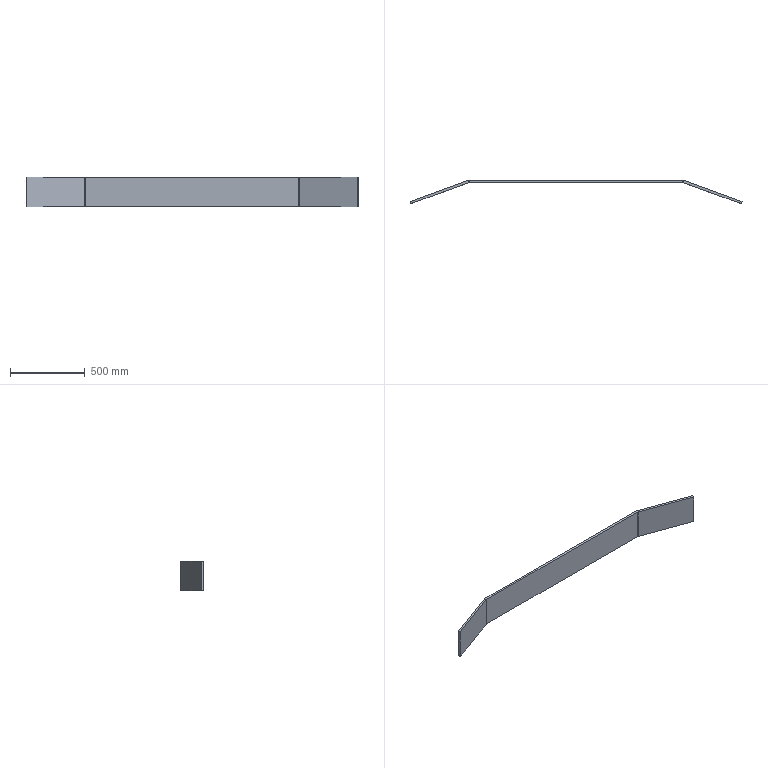Part | SolidWorks | features FlatPattern 1, SMBaseFlange 1, SheetMetal 1 | 1 solid | 22 faces | box 2215 x 156.912 x 200 mm | volume 7230328 mm3 | plane 18 | cylinder 4 | commonest cylinder face diameters 30 x2 62 x2
STEP:
#1=CARTESIAN_POINT('',(-717.485,-0.9046,200.));
#2=VERTEX_POINT('',#1);
#3=CARTESIAN_POINT('',(-722.958,14.13,200.));
#4=VERTEX_POINT('',#3);
#5=CARTESIAN_POINT('',(-717.485,-0.9046,200.));
#6=DIRECTION('',(-0.342,0.9397,0.));
#7=VECTOR('',#6,1000.);
#8=LINE('',#5,#7);
#9=EDGE_CURVE('',#2,#4,#8,.T.);
#10=ORIENTED_EDGE('',*,*,#9,.F.);
#11=CARTESIAN_POINT('',(-712.355,0.,200.));
#12=VERTEX_POINT('',#11);
#13=CARTESIAN_POINT('',(-712.355,-15.,200.));
#14=DIRECTION('',(0.,0.,-1.));
#15=DIRECTION('',(1.,0.,0.));
#16=AXIS2_PLACEMENT_3D('',#13,#14,#15);
#17=CIRCLE('',#16,15.);
#18=EDGE_CURVE('',#2,#12,#17,.T.);
#19=ORIENTED_EDGE('',*,*,#18,.T.);
#20=CARTESIAN_POINT('',(-712.355,16.,200.));
#21=VERTEX_POINT('',#20);
#22=CARTESIAN_POINT('',(-712.355,16.,200.));
#23=DIRECTION('',(0.,-1.,0.));
#24=VECTOR('',#23,1000.);
#25=LINE('',#22,#24);
#26=EDGE_CURVE('',#21,#12,#25,.T.);
#27=ORIENTED_EDGE('',*,*,#26,.F.);
#28=CARTESIAN_POINT('',(-712.355,-15.,200.));
#29=DIRECTION('',(0.,0.,-1.));
#30=DIRECTION('',(1.,0.,0.));
#31=AXIS2_PLACEMENT_3D('',#28,#29,#30);
#32=CIRCLE('',#31,31.);
#33=EDGE_CURVE('',#4,#21,#32,.T.);
#34=ORIENTED_EDGE('',*,*,#33,.F.);
#35=EDGE_LOOP('',(#10,#19,#27,#34));
#36=FACE_OUTER_BOUND('',#35,.T.);
#37=CARTESIAN_POINT('',(-717.485,-0.9046,200.));
#38=DIRECTION('',(0.,0.,1.));
#39=DIRECTION('',(1.,0.,0.));
#40=AXIS2_PLACEMENT_3D('',#37,#38,#39);
#41=PLANE('',#40);
#42=ADVANCED_FACE('',(#36),#41,.T.);
#43=CARTESIAN_POINT('',(-1102.153,-140.912,200.));
#44=VERTEX_POINT('',#43);
#45=CARTESIAN_POINT('',(-715.,0.,200.));
#46=DIRECTION('',(0.9397,0.342,0.));
#47=VECTOR('',#46,1000.);
#48=LINE('',#45,#47);
#49=EDGE_CURVE('',#44,#2,#48,.T.);
#50=ORIENTED_EDGE('',*,*,#49,.T.);
#51=ORIENTED_EDGE('',*,*,#9,.T.);
#52=CARTESIAN_POINT('',(-1107.626,-125.877,200.));
#53=VERTEX_POINT('',#52);
#54=CARTESIAN_POINT('',(-720.472,15.035,200.));
#55=DIRECTION('',(0.9397,0.342,0.));
#56=VECTOR('',#55,1000.);
#57=LINE('',#54,#56);
#58=EDGE_CURVE('',#53,#4,#57,.T.);
#59=ORIENTED_EDGE('',*,*,#58,.F.);
#60=CARTESIAN_POINT('',(-1102.153,-140.912,200.));
#61=DIRECTION('',(-0.342,0.9397,0.));
#62=VECTOR('',#61,1000.);
#63=LINE('',#60,#62);
#64=EDGE_CURVE('',#44,#53,#63,.T.);
#65=ORIENTED_EDGE('',*,*,#64,.F.);
#66=EDGE_LOOP('',(#50,#51,#59,#65));
#67=FACE_OUTER_BOUND('',#66,.T.);
#68=CARTESIAN_POINT('',(-712.355,16.,200.));
#69=DIRECTION('',(0.,0.,1.));
#70=DIRECTION('',(1.,0.,0.));
#71=AXIS2_PLACEMENT_3D('',#68,#69,#70);
#72=PLANE('',#71);
#73=ADVANCED_FACE('',(#67),#72,.T.);
#74=CARTESIAN_POINT('',(-712.355,0.,0.));
#75=VERTEX_POINT('',#74);
#76=CARTESIAN_POINT('',(-712.355,16.,0.));
#77=VERTEX_POINT('',#76);
#78=CARTESIAN_POINT('',(-712.355,0.,0.));
#79=DIRECTION('',(0.,1.,0.));
#80=VECTOR('',#79,1000.);
#81=LINE('',#78,#80);
#82=EDGE_CURVE('',#75,#77,#81,.T.);
#83=ORIENTED_EDGE('',*,*,#82,.F.);
#84=CARTESIAN_POINT('',(-717.485,-0.9046,0.));
#85=VERTEX_POINT('',#84);
#86=CARTESIAN_POINT('',(-712.355,-15.,0.));
#87=DIRECTION('',(0.,0.,-1.));
#88=DIRECTION('',(1.,0.,0.));
#89=AXIS2_PLACEMENT_3D('',#86,#87,#88);
#90=CIRCLE('',#89,15.);
#91=EDGE_CURVE('',#85,#75,#90,.T.);
#92=ORIENTED_EDGE('',*,*,#91,.F.);
#93=CARTESIAN_POINT('',(-722.958,14.13,0.));
#94=VERTEX_POINT('',#93);
#95=CARTESIAN_POINT('',(-722.958,14.13,0.));
#96=DIRECTION('',(0.342,-0.9397,0.));
#97=VECTOR('',#96,1000.);
#98=LINE('',#95,#97);
#99=EDGE_CURVE('',#94,#85,#98,.T.);
#100=ORIENTED_EDGE('',*,*,#99,.F.);
#101=CARTESIAN_POINT('',(-712.355,-15.,0.));
#102=DIRECTION('',(0.,0.,-1.));
#103=DIRECTION('',(1.,0.,0.));
#104=AXIS2_PLACEMENT_3D('',#101,#102,#103);
#105=CIRCLE('',#104,31.);
#106=EDGE_CURVE('',#94,#77,#105,.T.);
#107=ORIENTED_EDGE('',*,*,#106,.T.);
#108=EDGE_LOOP('',(#83,#92,#100,#107));
#109=FACE_OUTER_BOUND('',#108,.T.);
#110=CARTESIAN_POINT('',(-712.355,0.,0.));
#111=DIRECTION('',(0.,0.,-1.));
#112=DIRECTION('',(-1.,0.,0.));
#113=AXIS2_PLACEMENT_3D('',#110,#111,#112);
#114=PLANE('',#113);
#115=ADVANCED_FACE('',(#109),#114,.T.);
#116=CARTESIAN_POINT('',(712.355,0.,0.));
#117=VERTEX_POINT('',#116);
#118=CARTESIAN_POINT('',(-715.,0.,0.));
#119=DIRECTION('',(1.,0.,0.));
#120=VECTOR('',#119,1000.);
#121=LINE('',#118,#120);
#122=EDGE_CURVE('',#75,#117,#121,.T.);
#123=ORIENTED_EDGE('',*,*,#122,.F.);
#124=ORIENTED_EDGE('',*,*,#82,.T.);
#125=CARTESIAN_POINT('',(712.355,16.,0.));
#126=VERTEX_POINT('',#125);
#127=CARTESIAN_POINT('',(-715.,16.,0.));
#128=DIRECTION('',(1.,0.,0.));
#129=VECTOR('',#128,1000.);
#130=LINE('',#127,#129);
#131=EDGE_CURVE('',#77,#126,#130,.T.);
#132=ORIENTED_EDGE('',*,*,#131,.T.);
#133=CARTESIAN_POINT('',(712.355,16.,0.));
#134=DIRECTION('',(0.,-1.,0.));
#135=VECTOR('',#134,1000.);
#136=LINE('',#133,#135);
#137=EDGE_CURVE('',#126,#117,#136,.T.);
#138=ORIENTED_EDGE('',*,*,#137,.T.);
#139=EDGE_LOOP('',(#123,#124,#132,#138));
#140=FACE_OUTER_BOUND('',#139,.T.);
#141=CARTESIAN_POINT('',(-722.958,14.13,0.));
#142=DIRECTION('',(0.,0.,-1.));
#143=DIRECTION('',(-1.,0.,0.));
#144=AXIS2_PLACEMENT_3D('',#141,#142,#143);
#145=PLANE('',#144);
#146=ADVANCED_FACE('',(#140),#145,.T.);
#147=CARTESIAN_POINT('',(712.355,0.,200.));
#148=VERTEX_POINT('',#147);
#149=CARTESIAN_POINT('',(712.355,16.,200.));
#150=VERTEX_POINT('',#149);
#151=CARTESIAN_POINT('',(712.355,0.,200.));
#152=DIRECTION('',(0.,1.,0.));
#153=VECTOR('',#152,1000.);
#154=LINE('',#151,#153);
#155=EDGE_CURVE('',#148,#150,#154,.T.);
#156=ORIENTED_EDGE('',*,*,#155,.F.);
#157=CARTESIAN_POINT('',(717.485,-0.9046,200.));
#158=VERTEX_POINT('',#157);
#159=CARTESIAN_POINT('',(712.355,-15.,200.));
#160=DIRECTION('',(0.,0.,-1.));
#161=DIRECTION('',(1.,0.,0.));
#162=AXIS2_PLACEMENT_3D('',#159,#160,#161);
#163=CIRCLE('',#162,15.);
#164=EDGE_CURVE('',#148,#158,#163,.T.);
#165=ORIENTED_EDGE('',*,*,#164,.T.);
#166=CARTESIAN_POINT('',(722.958,14.13,200.));
#167=VERTEX_POINT('',#166);
#168=CARTESIAN_POINT('',(722.958,14.13,200.));
#169=DIRECTION('',(-0.342,-0.9397,0.));
#170=VECTOR('',#169,1000.);
#171=LINE('',#168,#170);
#172=EDGE_CURVE('',#167,#158,#171,.T.);
#173=ORIENTED_EDGE('',*,*,#172,.F.);
#174=CARTESIAN_POINT('',(712.355,-15.,200.));
#175=DIRECTION('',(0.,0.,-1.));
#176=DIRECTION('',(1.,0.,0.));
#177=AXIS2_PLACEMENT_3D('',#174,#175,#176);
#178=CIRCLE('',#177,31.);
#179=EDGE_CURVE('',#150,#167,#178,.T.);
#180=ORIENTED_EDGE('',*,*,#179,.F.);
#181=EDGE_LOOP('',(#156,#165,#173,#180));
#182=FACE_OUTER_BOUND('',#181,.T.);
#183=CARTESIAN_POINT('',(712.355,0.,200.));
#184=DIRECTION('',(0.,0.,1.));
#185=DIRECTION('',(1.,0.,0.));
#186=AXIS2_PLACEMENT_3D('',#183,#184,#185);
#187=PLANE('',#186);
#188=ADVANCED_FACE('',(#182),#187,.T.);
#189=CARTESIAN_POINT('',(-715.,0.,200.));
#190=DIRECTION('',(1.,0.,0.));
#191=VECTOR('',#190,1000.);
#192=LINE('',#189,#191);
#193=EDGE_CURVE('',#12,#148,#192,.T.);
#194=ORIENTED_EDGE('',*,*,#193,.T.);
#195=ORIENTED_EDGE('',*,*,#155,.T.);
#196=CARTESIAN_POINT('',(-715.,16.,200.));
#197=DIRECTION('',(1.,0.,0.));
#198=VECTOR('',#197,1000.);
#199=LINE('',#196,#198);
#200=EDGE_CURVE('',#21,#150,#199,.T.);
#201=ORIENTED_EDGE('',*,*,#200,.F.);
#202=ORIENTED_EDGE('',*,*,#26,.T.);
#203=EDGE_LOOP('',(#194,#195,#201,#202));
#204=FACE_OUTER_BOUND('',#203,.T.);
#205=CARTESIAN_POINT('',(722.958,14.13,200.));
#206=DIRECTION('',(0.,0.,1.));
#207=DIRECTION('',(1.,0.,0.));
#208=AXIS2_PLACEMENT_3D('',#205,#206,#207);
#209=PLANE('',#208);
#210=ADVANCED_FACE('',(#204),#209,.T.);
#211=CARTESIAN_POINT('',(717.485,-0.9046,0.));
#212=VERTEX_POINT('',#211);
#213=CARTESIAN_POINT('',(722.958,14.13,0.));
#214=VERTEX_POINT('',#213);
#215=CARTESIAN_POINT('',(717.485,-0.9046,0.));
#216=DIRECTION('',(0.342,0.9397,0.));
#217=VECTOR('',#216,1000.);
#218=LINE('',#215,#217);
#219=EDGE_CURVE('',#212,#214,#218,.T.);
#220=ORIENTED_EDGE('',*,*,#219,.F.);
#221=CARTESIAN_POINT('',(712.355,-15.,0.));
#222=DIRECTION('',(0.,0.,-1.));
#223=DIRECTION('',(1.,0.,0.));
#224=AXIS2_PLACEMENT_3D('',#221,#222,#223);
#225=CIRCLE('',#224,15.);
#226=EDGE_CURVE('',#117,#212,#225,.T.);
#227=ORIENTED_EDGE('',*,*,#226,.F.);
#228=ORIENTED_EDGE('',*,*,#137,.F.);
#229=CARTESIAN_POINT('',(712.355,-15.,0.));
#230=DIRECTION('',(0.,0.,-1.));
#231=DIRECTION('',(1.,0.,0.));
#232=AXIS2_PLACEMENT_3D('',#229,#230,#231);
#233=CIRCLE('',#232,31.);
#234=EDGE_CURVE('',#126,#214,#233,.T.);
#235=ORIENTED_EDGE('',*,*,#234,.T.);
#236=EDGE_LOOP('',(#220,#227,#228,#235));
#237=FACE_OUTER_BOUND('',#236,.T.);
#238=CARTESIAN_POINT('',(717.485,-0.9046,0.));
#239=DIRECTION('',(0.,0.,-1.));
#240=DIRECTION('',(-1.,0.,0.));
#241=AXIS2_PLACEMENT_3D('',#238,#239,#240);
#242=PLANE('',#241);
#243=ADVANCED_FACE('',(#237),#242,.T.);
#244=CARTESIAN_POINT('',(1102.153,-140.912,0.));
#245=VERTEX_POINT('',#244);
#246=CARTESIAN_POINT('',(715.,0.,0.));
#247=DIRECTION('',(0.9397,-0.342,0.));
#248=VECTOR('',#247,1000.);
#249=LINE('',#246,#248);
#250=EDGE_CURVE('',#212,#245,#249,.T.);
#251=ORIENTED_EDGE('',*,*,#250,.F.);
#252=ORIENTED_EDGE('',*,*,#219,.T.);
#253=CARTESIAN_POINT('',(1107.626,-125.877,0.));
#254=VERTEX_POINT('',#253);
#255=CARTESIAN_POINT('',(720.472,15.035,0.));
#256=DIRECTION('',(0.9397,-0.342,0.));
#257=VECTOR('',#256,1000.);
#258=LINE('',#255,#257);
#259=EDGE_CURVE('',#214,#254,#258,.T.);
#260=ORIENTED_EDGE('',*,*,#259,.T.);
#261=CARTESIAN_POINT('',(1107.626,-125.877,0.));
#262=DIRECTION('',(-0.342,-0.9397,0.));
#263=VECTOR('',#262,1000.);
#264=LINE('',#261,#263);
#265=EDGE_CURVE('',#254,#245,#264,.T.);
#266=ORIENTED_EDGE('',*,*,#265,.T.);
#267=EDGE_LOOP('',(#251,#252,#260,#266));
#268=FACE_OUTER_BOUND('',#267,.T.);
#269=CARTESIAN_POINT('',(712.355,16.,0.));
#270=DIRECTION('',(0.,0.,-1.));
#271=DIRECTION('',(-1.,0.,0.));
#272=AXIS2_PLACEMENT_3D('',#269,#270,#271);
#273=PLANE('',#272);
#274=ADVANCED_FACE('',(#268),#273,.T.);
#275=ORIENTED_EDGE('',*,*,#250,.T.);
#276=CARTESIAN_POINT('',(1102.153,-140.912,200.));
#277=VERTEX_POINT('',#276);
#278=CARTESIAN_POINT('',(1102.153,-140.912,200.));
#279=DIRECTION('',(0.,0.,-1.));
#280=VECTOR('',#279,1000.);
#281=LINE('',#278,#280);
#282=EDGE_CURVE('',#277,#245,#281,.T.);
#283=ORIENTED_EDGE('',*,*,#282,.F.);
#284=CARTESIAN_POINT('',(715.,0.,200.));
#285=DIRECTION('',(0.9397,-0.342,0.));
#286=VECTOR('',#285,1000.);
#287=LINE('',#284,#286);
#288=EDGE_CURVE('',#158,#277,#287,.T.);
#289=ORIENTED_EDGE('',*,*,#288,.F.);
#290=CARTESIAN_POINT('',(717.485,-0.9046,200.));
#291=DIRECTION('',(0.,0.,-1.));
#292=VECTOR('',#291,1000.);
#293=LINE('',#290,#292);
#294=EDGE_CURVE('',#158,#212,#293,.T.);
#295=ORIENTED_EDGE('',*,*,#294,.T.);
#296=EDGE_LOOP('',(#275,#283,#289,#295));
#297=FACE_OUTER_BOUND('',#296,.T.);
#298=CARTESIAN_POINT('',(715.,0.,200.));
#299=DIRECTION('',(0.342,0.9397,0.));
#300=DIRECTION('',(-0.9397,0.342,0.));
#301=AXIS2_PLACEMENT_3D('',#298,#299,#300);
#302=PLANE('',#301);
#303=ADVANCED_FACE('',(#297),#302,.F.);
#304=ORIENTED_EDGE('',*,*,#265,.F.);
#305=CARTESIAN_POINT('',(1107.626,-125.877,200.));
#306=VERTEX_POINT('',#305);
#307=CARTESIAN_POINT('',(1107.626,-125.877,200.));
#308=DIRECTION('',(0.,0.,-1.));
#309=VECTOR('',#308,1000.);
#310=LINE('',#307,#309);
#311=EDGE_CURVE('',#306,#254,#310,.T.);
#312=ORIENTED_EDGE('',*,*,#311,.F.);
#313=CARTESIAN_POINT('',(1107.626,-125.877,200.));
#314=DIRECTION('',(-0.342,-0.9397,0.));
#315=VECTOR('',#314,1000.);
#316=LINE('',#313,#315);
#317=EDGE_CURVE('',#306,#277,#316,.T.);
#318=ORIENTED_EDGE('',*,*,#317,.T.);
#319=ORIENTED_EDGE('',*,*,#282,.T.);
#320=EDGE_LOOP('',(#304,#312,#318,#319));
#321=FACE_OUTER_BOUND('',#320,.T.);
#322=CARTESIAN_POINT('',(1107.626,-125.877,200.));
#323=DIRECTION('',(0.9397,-0.342,0.));
#324=DIRECTION('',(0.342,0.9397,0.));
#325=AXIS2_PLACEMENT_3D('',#322,#323,#324);
#326=PLANE('',#325);
#327=ADVANCED_FACE('',(#321),#326,.T.);
#328=ORIENTED_EDGE('',*,*,#259,.F.);
#329=CARTESIAN_POINT('',(722.958,14.13,200.));
#330=DIRECTION('',(0.,0.,-1.));
#331=VECTOR('',#330,1000.);
#332=LINE('',#329,#331);
#333=EDGE_CURVE('',#167,#214,#332,.T.);
#334=ORIENTED_EDGE('',*,*,#333,.F.);
#335=CARTESIAN_POINT('',(720.472,15.035,200.));
#336=DIRECTION('',(0.9397,-0.342,0.));
#337=VECTOR('',#336,1000.);
#338=LINE('',#335,#337);
#339=EDGE_CURVE('',#167,#306,#338,.T.);
#340=ORIENTED_EDGE('',*,*,#339,.T.);
#341=ORIENTED_EDGE('',*,*,#311,.T.);
#342=EDGE_LOOP('',(#328,#334,#340,#341));
#343=FACE_OUTER_BOUND('',#342,.T.);
#344=CARTESIAN_POINT('',(720.472,15.035,200.));
#345=DIRECTION('',(0.342,0.9397,0.));
#346=DIRECTION('',(-0.9397,0.342,0.));
#347=AXIS2_PLACEMENT_3D('',#344,#345,#346);
#348=PLANE('',#347);
#349=ADVANCED_FACE('',(#343),#348,.T.);
#350=ORIENTED_EDGE('',*,*,#234,.F.);
#351=CARTESIAN_POINT('',(712.355,16.,200.));
#352=DIRECTION('',(0.,0.,-1.));
#353=VECTOR('',#352,1000.);
#354=LINE('',#351,#353);
#355=EDGE_CURVE('',#150,#126,#354,.T.);
#356=ORIENTED_EDGE('',*,*,#355,.F.);
#357=ORIENTED_EDGE('',*,*,#179,.T.);
#358=ORIENTED_EDGE('',*,*,#333,.T.);
#359=EDGE_LOOP('',(#350,#356,#357,#358));
#360=FACE_OUTER_BOUND('',#359,.T.);
#361=CARTESIAN_POINT('',(712.355,-15.,200.));
#362=DIRECTION('',(0.,0.,-1.));
#363=DIRECTION('',(-1.,0.,0.));
#364=AXIS2_PLACEMENT_3D('',#361,#362,#363);
#365=CYLINDRICAL_SURFACE('',#364,31.);
#366=ADVANCED_FACE('',(#360),#365,.T.);
#367=ORIENTED_EDGE('',*,*,#131,.F.);
#368=CARTESIAN_POINT('',(-712.355,16.,200.));
#369=DIRECTION('',(0.,0.,-1.));
#370=VECTOR('',#369,1000.);
#371=LINE('',#368,#370);
#372=EDGE_CURVE('',#21,#77,#371,.T.);
#373=ORIENTED_EDGE('',*,*,#372,.F.);
#374=ORIENTED_EDGE('',*,*,#200,.T.);
#375=ORIENTED_EDGE('',*,*,#355,.T.);
#376=EDGE_LOOP('',(#367,#373,#374,#375));
#377=FACE_OUTER_BOUND('',#376,.T.);
#378=CARTESIAN_POINT('',(-715.,16.,200.));
#379=DIRECTION('',(0.,1.,0.));
#380=DIRECTION('',(0.,0.,1.));
#381=AXIS2_PLACEMENT_3D('',#378,#379,#380);
#382=PLANE('',#381);
#383=ADVANCED_FACE('',(#377),#382,.T.);
#384=ORIENTED_EDGE('',*,*,#106,.F.);
#385=CARTESIAN_POINT('',(-722.958,14.13,200.));
#386=DIRECTION('',(0.,0.,-1.));
#387=VECTOR('',#386,1000.);
#388=LINE('',#385,#387);
#389=EDGE_CURVE('',#4,#94,#388,.T.);
#390=ORIENTED_EDGE('',*,*,#389,.F.);
#391=ORIENTED_EDGE('',*,*,#33,.T.);
#392=ORIENTED_EDGE('',*,*,#372,.T.);
#393=EDGE_LOOP('',(#384,#390,#391,#392));
#394=FACE_OUTER_BOUND('',#393,.T.);
#395=CARTESIAN_POINT('',(-712.355,-15.,200.));
#396=DIRECTION('',(0.,0.,-1.));
#397=DIRECTION('',(-1.,0.,0.));
#398=AXIS2_PLACEMENT_3D('',#395,#396,#397);
#399=CYLINDRICAL_SURFACE('',#398,31.);
#400=ADVANCED_FACE('',(#394),#399,.T.);
#401=CARTESIAN_POINT('',(-1107.626,-125.877,0.));
#402=VERTEX_POINT('',#401);
#403=CARTESIAN_POINT('',(-720.472,15.035,0.));
#404=DIRECTION('',(0.9397,0.342,0.));
#405=VECTOR('',#404,1000.);
#406=LINE('',#403,#405);
#407=EDGE_CURVE('',#402,#94,#406,.T.);
#408=ORIENTED_EDGE('',*,*,#407,.F.);
#409=CARTESIAN_POINT('',(-1107.626,-125.877,200.));
#410=DIRECTION('',(0.,0.,-1.));
#411=VECTOR('',#410,1000.);
#412=LINE('',#409,#411);
#413=EDGE_CURVE('',#53,#402,#412,.T.);
#414=ORIENTED_EDGE('',*,*,#413,.F.);
#415=ORIENTED_EDGE('',*,*,#58,.T.);
#416=ORIENTED_EDGE('',*,*,#389,.T.);
#417=EDGE_LOOP('',(#408,#414,#415,#416));
#418=FACE_OUTER_BOUND('',#417,.T.);
#419=CARTESIAN_POINT('',(-720.472,15.035,200.));
#420=DIRECTION('',(-0.342,0.9397,0.));
#421=DIRECTION('',(-0.9397,-0.342,0.));
#422=AXIS2_PLACEMENT_3D('',#419,#420,#421);
#423=PLANE('',#422);
#424=ADVANCED_FACE('',(#418),#423,.T.);
#425=CARTESIAN_POINT('',(-1102.153,-140.912,0.));
#426=VERTEX_POINT('',#425);
#427=CARTESIAN_POINT('',(-1102.153,-140.912,0.));
#428=DIRECTION('',(-0.342,0.9397,0.));
#429=VECTOR('',#428,1000.);
#430=LINE('',#427,#429);
#431=EDGE_CURVE('',#426,#402,#430,.T.);
#432=ORIENTED_EDGE('',*,*,#431,.F.);
#433=CARTESIAN_POINT('',(-1102.153,-140.912,200.));
#434=DIRECTION('',(0.,0.,-1.));
#435=VECTOR('',#434,1000.);
#436=LINE('',#433,#435);
#437=EDGE_CURVE('',#44,#426,#436,.T.);
#438=ORIENTED_EDGE('',*,*,#437,.F.);
#439=ORIENTED_EDGE('',*,*,#64,.T.);
#440=ORIENTED_EDGE('',*,*,#413,.T.);
#441=EDGE_LOOP('',(#432,#438,#439,#440));
#442=FACE_OUTER_BOUND('',#441,.T.);
#443=CARTESIAN_POINT('',(-1102.153,-140.912,200.));
#444=DIRECTION('',(-0.9397,-0.342,0.));
#445=DIRECTION('',(0.342,-0.9397,0.));
#446=AXIS2_PLACEMENT_3D('',#443,#444,#445);
#447=PLANE('',#446);
#448=ADVANCED_FACE('',(#442),#447,.T.);
#449=CARTESIAN_POINT('',(-715.,0.,0.));
#450=DIRECTION('',(0.9397,0.342,0.));
#451=VECTOR('',#450,1000.);
#452=LINE('',#449,#451);
#453=EDGE_CURVE('',#426,#85,#452,.T.);
#454=ORIENTED_EDGE('',*,*,#453,.T.);
#455=CARTESIAN_POINT('',(-717.485,-0.9046,200.));
#456=DIRECTION('',(0.,0.,-1.));
#457=VECTOR('',#456,1000.);
#458=LINE('',#455,#457);
#459=EDGE_CURVE('',#2,#85,#458,.T.);
#460=ORIENTED_EDGE('',*,*,#459,.F.);
#461=ORIENTED_EDGE('',*,*,#49,.F.);
#462=ORIENTED_EDGE('',*,*,#437,.T.);
#463=EDGE_LOOP('',(#454,#460,#461,#462));
#464=FACE_OUTER_BOUND('',#463,.T.);
#465=CARTESIAN_POINT('',(-715.,0.,200.));
#466=DIRECTION('',(-0.342,0.9397,0.));
#467=DIRECTION('',(-0.9397,-0.342,0.));
#468=AXIS2_PLACEMENT_3D('',#465,#466,#467);
#469=PLANE('',#468);
#470=ADVANCED_FACE('',(#464),#469,.F.);
#471=ORIENTED_EDGE('',*,*,#91,.T.);
#472=CARTESIAN_POINT('',(-712.355,0.,200.));
#473=DIRECTION('',(0.,0.,-1.));
#474=VECTOR('',#473,1000.);
#475=LINE('',#472,#474);
#476=EDGE_CURVE('',#12,#75,#475,.T.);
#477=ORIENTED_EDGE('',*,*,#476,.F.);
#478=ORIENTED_EDGE('',*,*,#18,.F.);
#479=ORIENTED_EDGE('',*,*,#459,.T.);
#480=EDGE_LOOP('',(#471,#477,#478,#479));
#481=FACE_OUTER_BOUND('',#480,.T.);
#482=CARTESIAN_POINT('',(-712.355,-15.,200.));
#483=DIRECTION('',(0.,0.,-1.));
#484=DIRECTION('',(-1.,0.,0.));
#485=AXIS2_PLACEMENT_3D('',#482,#483,#484);
#486=CYLINDRICAL_SURFACE('',#485,15.);
#487=ADVANCED_FACE('',(#481),#486,.F.);
#488=ORIENTED_EDGE('',*,*,#122,.T.);
#489=CARTESIAN_POINT('',(712.355,0.,200.));
#490=DIRECTION('',(0.,0.,-1.));
#491=VECTOR('',#490,1000.);
#492=LINE('',#489,#491);
#493=EDGE_CURVE('',#148,#117,#492,.T.);
#494=ORIENTED_EDGE('',*,*,#493,.F.);
#495=ORIENTED_EDGE('',*,*,#193,.F.);
#496=ORIENTED_EDGE('',*,*,#476,.T.);
#497=EDGE_LOOP('',(#488,#494,#495,#496));
#498=FACE_OUTER_BOUND('',#497,.T.);
#499=CARTESIAN_POINT('',(-715.,0.,200.));
#500=DIRECTION('',(0.,1.,0.));
#501=DIRECTION('',(0.,0.,1.));
#502=AXIS2_PLACEMENT_3D('',#499,#500,#501);
#503=PLANE('',#502);
#504=ADVANCED_FACE('',(#498),#503,.F.);
#505=ORIENTED_EDGE('',*,*,#226,.T.);
#506=ORIENTED_EDGE('',*,*,#294,.F.);
#507=ORIENTED_EDGE('',*,*,#164,.F.);
#508=ORIENTED_EDGE('',*,*,#493,.T.);
#509=EDGE_LOOP('',(#505,#506,#507,#508));
#510=FACE_OUTER_BOUND('',#509,.T.);
#511=CARTESIAN_POINT('',(712.355,-15.,200.));
#512=DIRECTION('',(0.,0.,-1.));
#513=DIRECTION('',(-1.,0.,0.));
#514=AXIS2_PLACEMENT_3D('',#511,#512,#513);
#515=CYLINDRICAL_SURFACE('',#514,15.);
#516=ADVANCED_FACE('',(#510),#515,.F.);
#517=ORIENTED_EDGE('',*,*,#288,.T.);
#518=ORIENTED_EDGE('',*,*,#317,.F.);
#519=ORIENTED_EDGE('',*,*,#339,.F.);
#520=ORIENTED_EDGE('',*,*,#172,.T.);
#521=EDGE_LOOP('',(#517,#518,#519,#520));
#522=FACE_OUTER_BOUND('',#521,.T.);
#523=CARTESIAN_POINT('',(712.355,-15.,200.));
#524=DIRECTION('',(0.,0.,1.));
#525=DIRECTION('',(1.,0.,0.));
#526=AXIS2_PLACEMENT_3D('',#523,#524,#525);
#527=PLANE('',#526);
#528=ADVANCED_FACE('',(#522),#527,.T.);
#529=ORIENTED_EDGE('',*,*,#407,.T.);
#530=ORIENTED_EDGE('',*,*,#99,.T.);
#531=ORIENTED_EDGE('',*,*,#453,.F.);
#532=ORIENTED_EDGE('',*,*,#431,.T.);
#533=EDGE_LOOP('',(#529,#530,#531,#532));
#534=FACE_OUTER_BOUND('',#533,.T.);
#535=CARTESIAN_POINT('',(712.355,-15.,0.));
#536=DIRECTION('',(0.,0.,1.));
#537=DIRECTION('',(1.,0.,0.));
#538=AXIS2_PLACEMENT_3D('',#535,#536,#537);
#539=PLANE('',#538);
#540=ADVANCED_FACE('',(#534),#539,.F.);
#541=CLOSED_SHELL('',(#42,#73,#115,#146,#188,#210,#243,#274,#303,#327,#349,#366,#383,#400,#424,#448,#470,#487,#504,#516,#528,#540));
#542=MANIFOLD_SOLID_BREP('',#541);
#543=CARTESIAN_POINT('',(0.,0.,0.));
#544=DIRECTION('',(0.,0.,1.));
#545=DIRECTION('',(1.,0.,0.));
#546=AXIS2_PLACEMENT_3D('',#543,#544,#545);
#547=(LENGTH_UNIT()NAMED_UNIT(*)SI_UNIT(.MILLI.,.METRE.));
#548=UNCERTAINTY_MEASURE_WITH_UNIT(LENGTH_MEASURE(0.00001),#547,'','');
#549=(NAMED_UNIT(*)PLANE_ANGLE_UNIT()SI_UNIT($,.RADIAN.));
#550=(NAMED_UNIT(*)SI_UNIT($,.STERADIAN.)SOLID_ANGLE_UNIT());
#551=(GEOMETRIC_REPRESENTATION_CONTEXT(3)GLOBAL_UNCERTAINTY_ASSIGNED_CONTEXT((#548))GLOBAL_UNIT_ASSIGNED_CONTEXT((#547,#549,#550))REPRESENTATION_CONTEXT('',''));
#552=ADVANCED_BREP_SHAPE_REPRESENTATION('',(#542,#546),#551);